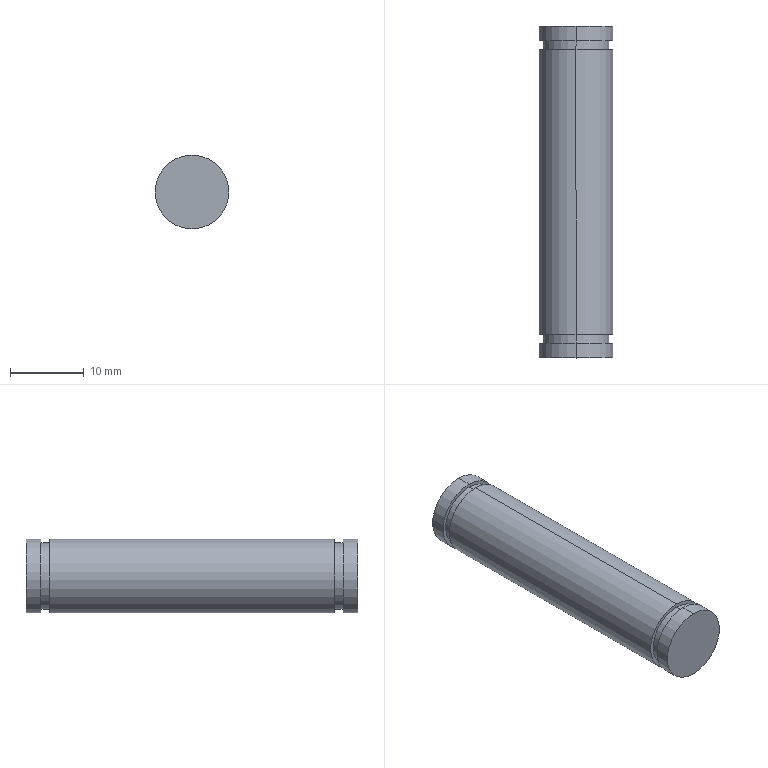Part | SolidWorks | features Revolution 1 | 1 solid | 16 faces | box 10 x 45 x 10 mm | volume 3498 mm3 | cylinder 10 | plane 6 | commonest cylinder face diameters 10 x6 9 x4
STEP:
#1=CARTESIAN_POINT('',(0.,-20.5,4.5));
#2=VERTEX_POINT('',#1);
#3=CARTESIAN_POINT('',(0.,-20.5,-4.5));
#4=VERTEX_POINT('',#3);
#5=CARTESIAN_POINT('',(0.,-20.5,0.));
#6=DIRECTION('',(0.,1.,0.));
#7=DIRECTION('',(0.,0.,1.));
#8=AXIS2_PLACEMENT_3D('',#5,#6,#7);
#9=CIRCLE('',#8,4.5);
#10=EDGE_CURVE('',#2,#4,#9,.T.);
#11=ORIENTED_EDGE('',*,*,#10,.T.);
#12=CARTESIAN_POINT('',(0.,-19.3,-4.5));
#13=VERTEX_POINT('',#12);
#14=CARTESIAN_POINT('',(0.,-22.5,-4.5));
#15=DIRECTION('',(0.,1.,0.));
#16=VECTOR('',#15,1000.);
#17=LINE('',#14,#16);
#18=EDGE_CURVE('',#4,#13,#17,.T.);
#19=ORIENTED_EDGE('',*,*,#18,.T.);
#20=CARTESIAN_POINT('',(0.,-19.3,4.5));
#21=VERTEX_POINT('',#20);
#22=CARTESIAN_POINT('',(0.,-19.3,0.));
#23=DIRECTION('',(0.,1.,0.));
#24=DIRECTION('',(0.,0.,1.));
#25=AXIS2_PLACEMENT_3D('',#22,#23,#24);
#26=CIRCLE('',#25,4.5);
#27=EDGE_CURVE('',#21,#13,#26,.T.);
#28=ORIENTED_EDGE('',*,*,#27,.F.);
#29=CARTESIAN_POINT('',(0.,-22.5,4.5));
#30=DIRECTION('',(0.,1.,0.));
#31=VECTOR('',#30,1000.);
#32=LINE('',#29,#31);
#33=EDGE_CURVE('',#2,#21,#32,.T.);
#34=ORIENTED_EDGE('',*,*,#33,.F.);
#35=EDGE_LOOP('',(#11,#19,#28,#34));
#36=FACE_OUTER_BOUND('',#35,.T.);
#37=CARTESIAN_POINT('',(0.,-22.5,0.));
#38=DIRECTION('',(0.,1.,0.));
#39=DIRECTION('',(0.,0.,1.));
#40=AXIS2_PLACEMENT_3D('',#37,#38,#39);
#41=CYLINDRICAL_SURFACE('',#40,4.5);
#42=ADVANCED_FACE('',(#36),#41,.T.);
#43=CARTESIAN_POINT('',(0.,-19.3,5.));
#44=VERTEX_POINT('',#43);
#45=CARTESIAN_POINT('',(0.,-19.3,-5.));
#46=VERTEX_POINT('',#45);
#47=CARTESIAN_POINT('',(0.,-19.3,0.));
#48=DIRECTION('',(0.,1.,0.));
#49=DIRECTION('',(0.,0.,1.));
#50=AXIS2_PLACEMENT_3D('',#47,#48,#49);
#51=CIRCLE('',#50,5.);
#52=EDGE_CURVE('',#44,#46,#51,.T.);
#53=ORIENTED_EDGE('',*,*,#52,.T.);
#54=CARTESIAN_POINT('',(0.,19.3,-5.));
#55=VERTEX_POINT('',#54);
#56=CARTESIAN_POINT('',(0.,-22.5,-5.));
#57=DIRECTION('',(0.,1.,0.));
#58=VECTOR('',#57,1000.);
#59=LINE('',#56,#58);
#60=EDGE_CURVE('',#46,#55,#59,.T.);
#61=ORIENTED_EDGE('',*,*,#60,.T.);
#62=CARTESIAN_POINT('',(0.,19.3,5.));
#63=VERTEX_POINT('',#62);
#64=CARTESIAN_POINT('',(0.,19.3,0.));
#65=DIRECTION('',(0.,1.,0.));
#66=DIRECTION('',(0.,0.,1.));
#67=AXIS2_PLACEMENT_3D('',#64,#65,#66);
#68=CIRCLE('',#67,5.);
#69=EDGE_CURVE('',#63,#55,#68,.T.);
#70=ORIENTED_EDGE('',*,*,#69,.F.);
#71=CARTESIAN_POINT('',(0.,-22.5,5.));
#72=DIRECTION('',(0.,1.,0.));
#73=VECTOR('',#72,1000.);
#74=LINE('',#71,#73);
#75=EDGE_CURVE('',#44,#63,#74,.T.);
#76=ORIENTED_EDGE('',*,*,#75,.F.);
#77=EDGE_LOOP('',(#53,#61,#70,#76));
#78=FACE_OUTER_BOUND('',#77,.T.);
#79=CARTESIAN_POINT('',(0.,-22.5,0.));
#80=DIRECTION('',(0.,1.,0.));
#81=DIRECTION('',(0.,0.,1.));
#82=AXIS2_PLACEMENT_3D('',#79,#80,#81);
#83=CYLINDRICAL_SURFACE('',#82,5.);
#84=ADVANCED_FACE('',(#78),#83,.T.);
#85=CARTESIAN_POINT('',(0.,19.3,4.5));
#86=VERTEX_POINT('',#85);
#87=CARTESIAN_POINT('',(0.,19.3,-4.5));
#88=VERTEX_POINT('',#87);
#89=CARTESIAN_POINT('',(0.,19.3,0.));
#90=DIRECTION('',(0.,1.,0.));
#91=DIRECTION('',(0.,0.,1.));
#92=AXIS2_PLACEMENT_3D('',#89,#90,#91);
#93=CIRCLE('',#92,4.5);
#94=EDGE_CURVE('',#86,#88,#93,.T.);
#95=ORIENTED_EDGE('',*,*,#94,.T.);
#96=CARTESIAN_POINT('',(0.,20.5,-4.5));
#97=VERTEX_POINT('',#96);
#98=CARTESIAN_POINT('',(0.,-22.5,-4.5));
#99=DIRECTION('',(0.,1.,0.));
#100=VECTOR('',#99,1000.);
#101=LINE('',#98,#100);
#102=EDGE_CURVE('',#88,#97,#101,.T.);
#103=ORIENTED_EDGE('',*,*,#102,.T.);
#104=CARTESIAN_POINT('',(0.,20.5,4.5));
#105=VERTEX_POINT('',#104);
#106=CARTESIAN_POINT('',(0.,20.5,0.));
#107=DIRECTION('',(0.,1.,0.));
#108=DIRECTION('',(0.,0.,1.));
#109=AXIS2_PLACEMENT_3D('',#106,#107,#108);
#110=CIRCLE('',#109,4.5);
#111=EDGE_CURVE('',#105,#97,#110,.T.);
#112=ORIENTED_EDGE('',*,*,#111,.F.);
#113=CARTESIAN_POINT('',(0.,-22.5,4.5));
#114=DIRECTION('',(0.,1.,0.));
#115=VECTOR('',#114,1000.);
#116=LINE('',#113,#115);
#117=EDGE_CURVE('',#86,#105,#116,.T.);
#118=ORIENTED_EDGE('',*,*,#117,.F.);
#119=EDGE_LOOP('',(#95,#103,#112,#118));
#120=FACE_OUTER_BOUND('',#119,.T.);
#121=CARTESIAN_POINT('',(0.,-22.5,0.));
#122=DIRECTION('',(0.,1.,0.));
#123=DIRECTION('',(0.,0.,1.));
#124=AXIS2_PLACEMENT_3D('',#121,#122,#123);
#125=CYLINDRICAL_SURFACE('',#124,4.5);
#126=ADVANCED_FACE('',(#120),#125,.T.);
#127=CARTESIAN_POINT('',(0.,20.5,5.));
#128=VERTEX_POINT('',#127);
#129=CARTESIAN_POINT('',(0.,20.5,-5.));
#130=VERTEX_POINT('',#129);
#131=CARTESIAN_POINT('',(0.,20.5,0.));
#132=DIRECTION('',(0.,1.,0.));
#133=DIRECTION('',(0.,0.,1.));
#134=AXIS2_PLACEMENT_3D('',#131,#132,#133);
#135=CIRCLE('',#134,5.);
#136=EDGE_CURVE('',#128,#130,#135,.T.);
#137=ORIENTED_EDGE('',*,*,#136,.T.);
#138=CARTESIAN_POINT('',(0.,22.5,-5.));
#139=VERTEX_POINT('',#138);
#140=CARTESIAN_POINT('',(0.,-22.5,-5.));
#141=DIRECTION('',(0.,1.,0.));
#142=VECTOR('',#141,1000.);
#143=LINE('',#140,#142);
#144=EDGE_CURVE('',#130,#139,#143,.T.);
#145=ORIENTED_EDGE('',*,*,#144,.T.);
#146=CARTESIAN_POINT('',(0.,22.5,5.));
#147=VERTEX_POINT('',#146);
#148=CARTESIAN_POINT('',(0.,22.5,0.));
#149=DIRECTION('',(0.,1.,0.));
#150=DIRECTION('',(0.,0.,1.));
#151=AXIS2_PLACEMENT_3D('',#148,#149,#150);
#152=CIRCLE('',#151,5.);
#153=EDGE_CURVE('',#147,#139,#152,.T.);
#154=ORIENTED_EDGE('',*,*,#153,.F.);
#155=CARTESIAN_POINT('',(0.,-22.5,5.));
#156=DIRECTION('',(0.,1.,0.));
#157=VECTOR('',#156,1000.);
#158=LINE('',#155,#157);
#159=EDGE_CURVE('',#128,#147,#158,.T.);
#160=ORIENTED_EDGE('',*,*,#159,.F.);
#161=EDGE_LOOP('',(#137,#145,#154,#160));
#162=FACE_OUTER_BOUND('',#161,.T.);
#163=CARTESIAN_POINT('',(0.,-22.5,0.));
#164=DIRECTION('',(0.,1.,0.));
#165=DIRECTION('',(0.,0.,1.));
#166=AXIS2_PLACEMENT_3D('',#163,#164,#165);
#167=CYLINDRICAL_SURFACE('',#166,5.);
#168=ADVANCED_FACE('',(#162),#167,.T.);
#169=CARTESIAN_POINT('',(0.,-22.5,5.));
#170=VERTEX_POINT('',#169);
#171=CARTESIAN_POINT('',(0.,-22.5,-5.));
#172=VERTEX_POINT('',#171);
#173=CARTESIAN_POINT('',(0.,-22.5,0.));
#174=DIRECTION('',(0.,1.,0.));
#175=DIRECTION('',(0.,0.,1.));
#176=AXIS2_PLACEMENT_3D('',#173,#174,#175);
#177=CIRCLE('',#176,5.);
#178=EDGE_CURVE('',#170,#172,#177,.T.);
#179=ORIENTED_EDGE('',*,*,#178,.T.);
#180=CARTESIAN_POINT('',(0.,-20.5,-5.));
#181=VERTEX_POINT('',#180);
#182=CARTESIAN_POINT('',(0.,-22.5,-5.));
#183=DIRECTION('',(0.,1.,0.));
#184=VECTOR('',#183,1000.);
#185=LINE('',#182,#184);
#186=EDGE_CURVE('',#172,#181,#185,.T.);
#187=ORIENTED_EDGE('',*,*,#186,.T.);
#188=CARTESIAN_POINT('',(0.,-20.5,5.));
#189=VERTEX_POINT('',#188);
#190=CARTESIAN_POINT('',(0.,-20.5,0.));
#191=DIRECTION('',(0.,1.,0.));
#192=DIRECTION('',(0.,0.,1.));
#193=AXIS2_PLACEMENT_3D('',#190,#191,#192);
#194=CIRCLE('',#193,5.);
#195=EDGE_CURVE('',#189,#181,#194,.T.);
#196=ORIENTED_EDGE('',*,*,#195,.F.);
#197=CARTESIAN_POINT('',(0.,-22.5,5.));
#198=DIRECTION('',(0.,1.,0.));
#199=VECTOR('',#198,1000.);
#200=LINE('',#197,#199);
#201=EDGE_CURVE('',#170,#189,#200,.T.);
#202=ORIENTED_EDGE('',*,*,#201,.F.);
#203=EDGE_LOOP('',(#179,#187,#196,#202));
#204=FACE_OUTER_BOUND('',#203,.T.);
#205=CARTESIAN_POINT('',(0.,-22.5,0.));
#206=DIRECTION('',(0.,1.,0.));
#207=DIRECTION('',(0.,0.,1.));
#208=AXIS2_PLACEMENT_3D('',#205,#206,#207);
#209=CYLINDRICAL_SURFACE('',#208,5.);
#210=ADVANCED_FACE('',(#204),#209,.T.);
#211=ORIENTED_EDGE('',*,*,#186,.F.);
#212=CARTESIAN_POINT('',(0.,-22.5,0.));
#213=DIRECTION('',(0.,1.,0.));
#214=DIRECTION('',(0.,0.,1.));
#215=AXIS2_PLACEMENT_3D('',#212,#213,#214);
#216=CIRCLE('',#215,5.);
#217=EDGE_CURVE('',#172,#170,#216,.T.);
#218=ORIENTED_EDGE('',*,*,#217,.T.);
#219=ORIENTED_EDGE('',*,*,#201,.T.);
#220=CARTESIAN_POINT('',(0.,-20.5,0.));
#221=DIRECTION('',(0.,1.,0.));
#222=DIRECTION('',(0.,0.,1.));
#223=AXIS2_PLACEMENT_3D('',#220,#221,#222);
#224=CIRCLE('',#223,5.);
#225=EDGE_CURVE('',#181,#189,#224,.T.);
#226=ORIENTED_EDGE('',*,*,#225,.F.);
#227=EDGE_LOOP('',(#211,#218,#219,#226));
#228=FACE_OUTER_BOUND('',#227,.T.);
#229=CARTESIAN_POINT('',(0.,-22.5,0.));
#230=DIRECTION('',(0.,1.,0.));
#231=DIRECTION('',(0.,0.,1.));
#232=AXIS2_PLACEMENT_3D('',#229,#230,#231);
#233=CYLINDRICAL_SURFACE('',#232,5.);
#234=ADVANCED_FACE('',(#228),#233,.T.);
#235=ORIENTED_EDGE('',*,*,#178,.F.);
#236=ORIENTED_EDGE('',*,*,#217,.F.);
#237=EDGE_LOOP('',(#235,#236));
#238=FACE_OUTER_BOUND('',#237,.T.);
#239=CARTESIAN_POINT('',(5.,-22.5,0.));
#240=DIRECTION('',(0.,-1.,0.));
#241=DIRECTION('',(0.,0.,-1.));
#242=AXIS2_PLACEMENT_3D('',#239,#240,#241);
#243=PLANE('',#242);
#244=ADVANCED_FACE('',(#238),#243,.T.);
#245=ORIENTED_EDGE('',*,*,#153,.T.);
#246=CARTESIAN_POINT('',(0.,22.5,0.));
#247=DIRECTION('',(0.,1.,0.));
#248=DIRECTION('',(0.,0.,1.));
#249=AXIS2_PLACEMENT_3D('',#246,#247,#248);
#250=CIRCLE('',#249,5.);
#251=EDGE_CURVE('',#139,#147,#250,.T.);
#252=ORIENTED_EDGE('',*,*,#251,.T.);
#253=EDGE_LOOP('',(#245,#252));
#254=FACE_OUTER_BOUND('',#253,.T.);
#255=CARTESIAN_POINT('',(0.,22.5,0.));
#256=DIRECTION('',(0.,1.,0.));
#257=DIRECTION('',(0.,0.,1.));
#258=AXIS2_PLACEMENT_3D('',#255,#256,#257);
#259=PLANE('',#258);
#260=ADVANCED_FACE('',(#254),#259,.T.);
#261=ORIENTED_EDGE('',*,*,#144,.F.);
#262=CARTESIAN_POINT('',(0.,20.5,0.));
#263=DIRECTION('',(0.,1.,0.));
#264=DIRECTION('',(0.,0.,1.));
#265=AXIS2_PLACEMENT_3D('',#262,#263,#264);
#266=CIRCLE('',#265,5.);
#267=EDGE_CURVE('',#130,#128,#266,.T.);
#268=ORIENTED_EDGE('',*,*,#267,.T.);
#269=ORIENTED_EDGE('',*,*,#159,.T.);
#270=ORIENTED_EDGE('',*,*,#251,.F.);
#271=EDGE_LOOP('',(#261,#268,#269,#270));
#272=FACE_OUTER_BOUND('',#271,.T.);
#273=CARTESIAN_POINT('',(0.,-22.5,0.));
#274=DIRECTION('',(0.,1.,0.));
#275=DIRECTION('',(0.,0.,1.));
#276=AXIS2_PLACEMENT_3D('',#273,#274,#275);
#277=CYLINDRICAL_SURFACE('',#276,5.);
#278=ADVANCED_FACE('',(#272),#277,.T.);
#279=ORIENTED_EDGE('',*,*,#111,.T.);
#280=CARTESIAN_POINT('',(0.,20.5,0.));
#281=DIRECTION('',(0.,1.,0.));
#282=DIRECTION('',(0.,0.,1.));
#283=AXIS2_PLACEMENT_3D('',#280,#281,#282);
#284=CIRCLE('',#283,4.5);
#285=EDGE_CURVE('',#97,#105,#284,.T.);
#286=ORIENTED_EDGE('',*,*,#285,.T.);
#287=EDGE_LOOP('',(#279,#286));
#288=FACE_BOUND('',#287,.T.);
#289=ORIENTED_EDGE('',*,*,#136,.F.);
#290=ORIENTED_EDGE('',*,*,#267,.F.);
#291=EDGE_LOOP('',(#289,#290));
#292=FACE_OUTER_BOUND('',#291,.T.);
#293=CARTESIAN_POINT('',(5.,20.5,0.));
#294=DIRECTION('',(0.,-1.,0.));
#295=DIRECTION('',(0.,0.,-1.));
#296=AXIS2_PLACEMENT_3D('',#293,#294,#295);
#297=PLANE('',#296);
#298=ADVANCED_FACE('',(#288,#292),#297,.T.);
#299=ORIENTED_EDGE('',*,*,#102,.F.);
#300=CARTESIAN_POINT('',(0.,19.3,0.));
#301=DIRECTION('',(0.,1.,0.));
#302=DIRECTION('',(0.,0.,1.));
#303=AXIS2_PLACEMENT_3D('',#300,#301,#302);
#304=CIRCLE('',#303,4.5);
#305=EDGE_CURVE('',#88,#86,#304,.T.);
#306=ORIENTED_EDGE('',*,*,#305,.T.);
#307=ORIENTED_EDGE('',*,*,#117,.T.);
#308=ORIENTED_EDGE('',*,*,#285,.F.);
#309=EDGE_LOOP('',(#299,#306,#307,#308));
#310=FACE_OUTER_BOUND('',#309,.T.);
#311=CARTESIAN_POINT('',(0.,-22.5,0.));
#312=DIRECTION('',(0.,1.,0.));
#313=DIRECTION('',(0.,0.,1.));
#314=AXIS2_PLACEMENT_3D('',#311,#312,#313);
#315=CYLINDRICAL_SURFACE('',#314,4.5);
#316=ADVANCED_FACE('',(#310),#315,.T.);
#317=ORIENTED_EDGE('',*,*,#69,.T.);
#318=CARTESIAN_POINT('',(0.,19.3,0.));
#319=DIRECTION('',(0.,1.,0.));
#320=DIRECTION('',(0.,0.,1.));
#321=AXIS2_PLACEMENT_3D('',#318,#319,#320);
#322=CIRCLE('',#321,5.);
#323=EDGE_CURVE('',#55,#63,#322,.T.);
#324=ORIENTED_EDGE('',*,*,#323,.T.);
#325=EDGE_LOOP('',(#317,#324));
#326=FACE_OUTER_BOUND('',#325,.T.);
#327=ORIENTED_EDGE('',*,*,#94,.F.);
#328=ORIENTED_EDGE('',*,*,#305,.F.);
#329=EDGE_LOOP('',(#327,#328));
#330=FACE_BOUND('',#329,.T.);
#331=CARTESIAN_POINT('',(4.5,19.3,0.));
#332=DIRECTION('',(0.,1.,0.));
#333=DIRECTION('',(0.,0.,1.));
#334=AXIS2_PLACEMENT_3D('',#331,#332,#333);
#335=PLANE('',#334);
#336=ADVANCED_FACE('',(#326,#330),#335,.T.);
#337=ORIENTED_EDGE('',*,*,#60,.F.);
#338=CARTESIAN_POINT('',(0.,-19.3,0.));
#339=DIRECTION('',(0.,1.,0.));
#340=DIRECTION('',(0.,0.,1.));
#341=AXIS2_PLACEMENT_3D('',#338,#339,#340);
#342=CIRCLE('',#341,5.);
#343=EDGE_CURVE('',#46,#44,#342,.T.);
#344=ORIENTED_EDGE('',*,*,#343,.T.);
#345=ORIENTED_EDGE('',*,*,#75,.T.);
#346=ORIENTED_EDGE('',*,*,#323,.F.);
#347=EDGE_LOOP('',(#337,#344,#345,#346));
#348=FACE_OUTER_BOUND('',#347,.T.);
#349=CARTESIAN_POINT('',(0.,-22.5,0.));
#350=DIRECTION('',(0.,1.,0.));
#351=DIRECTION('',(0.,0.,1.));
#352=AXIS2_PLACEMENT_3D('',#349,#350,#351);
#353=CYLINDRICAL_SURFACE('',#352,5.);
#354=ADVANCED_FACE('',(#348),#353,.T.);
#355=ORIENTED_EDGE('',*,*,#27,.T.);
#356=CARTESIAN_POINT('',(0.,-19.3,0.));
#357=DIRECTION('',(0.,1.,0.));
#358=DIRECTION('',(0.,0.,1.));
#359=AXIS2_PLACEMENT_3D('',#356,#357,#358);
#360=CIRCLE('',#359,4.5);
#361=EDGE_CURVE('',#13,#21,#360,.T.);
#362=ORIENTED_EDGE('',*,*,#361,.T.);
#363=EDGE_LOOP('',(#355,#362));
#364=FACE_BOUND('',#363,.T.);
#365=ORIENTED_EDGE('',*,*,#52,.F.);
#366=ORIENTED_EDGE('',*,*,#343,.F.);
#367=EDGE_LOOP('',(#365,#366));
#368=FACE_OUTER_BOUND('',#367,.T.);
#369=CARTESIAN_POINT('',(5.,-19.3,0.));
#370=DIRECTION('',(0.,-1.,0.));
#371=DIRECTION('',(0.,0.,-1.));
#372=AXIS2_PLACEMENT_3D('',#369,#370,#371);
#373=PLANE('',#372);
#374=ADVANCED_FACE('',(#364,#368),#373,.T.);
#375=ORIENTED_EDGE('',*,*,#18,.F.);
#376=CARTESIAN_POINT('',(0.,-20.5,0.));
#377=DIRECTION('',(0.,1.,0.));
#378=DIRECTION('',(0.,0.,1.));
#379=AXIS2_PLACEMENT_3D('',#376,#377,#378);
#380=CIRCLE('',#379,4.5);
#381=EDGE_CURVE('',#4,#2,#380,.T.);
#382=ORIENTED_EDGE('',*,*,#381,.T.);
#383=ORIENTED_EDGE('',*,*,#33,.T.);
#384=ORIENTED_EDGE('',*,*,#361,.F.);
#385=EDGE_LOOP('',(#375,#382,#383,#384));
#386=FACE_OUTER_BOUND('',#385,.T.);
#387=CARTESIAN_POINT('',(0.,-22.5,0.));
#388=DIRECTION('',(0.,1.,0.));
#389=DIRECTION('',(0.,0.,1.));
#390=AXIS2_PLACEMENT_3D('',#387,#388,#389);
#391=CYLINDRICAL_SURFACE('',#390,4.5);
#392=ADVANCED_FACE('',(#386),#391,.T.);
#393=ORIENTED_EDGE('',*,*,#195,.T.);
#394=ORIENTED_EDGE('',*,*,#225,.T.);
#395=EDGE_LOOP('',(#393,#394));
#396=FACE_OUTER_BOUND('',#395,.T.);
#397=ORIENTED_EDGE('',*,*,#10,.F.);
#398=ORIENTED_EDGE('',*,*,#381,.F.);
#399=EDGE_LOOP('',(#397,#398));
#400=FACE_BOUND('',#399,.T.);
#401=CARTESIAN_POINT('',(4.5,-20.5,0.));
#402=DIRECTION('',(0.,1.,0.));
#403=DIRECTION('',(0.,0.,1.));
#404=AXIS2_PLACEMENT_3D('',#401,#402,#403);
#405=PLANE('',#404);
#406=ADVANCED_FACE('',(#396,#400),#405,.T.);
#407=CLOSED_SHELL('',(#42,#84,#126,#168,#210,#234,#244,#260,#278,#298,#316,#336,#354,#374,#392,#406));
#408=MANIFOLD_SOLID_BREP('',#407);
#409=CARTESIAN_POINT('',(0.,0.,0.));
#410=DIRECTION('',(0.,0.,1.));
#411=DIRECTION('',(1.,0.,0.));
#412=AXIS2_PLACEMENT_3D('',#409,#410,#411);
#413=(LENGTH_UNIT()NAMED_UNIT(*)SI_UNIT(.MILLI.,.METRE.));
#414=UNCERTAINTY_MEASURE_WITH_UNIT(LENGTH_MEASURE(0.00001),#413,'','');
#415=(NAMED_UNIT(*)PLANE_ANGLE_UNIT()SI_UNIT($,.RADIAN.));
#416=(NAMED_UNIT(*)SI_UNIT($,.STERADIAN.)SOLID_ANGLE_UNIT());
#417=(GEOMETRIC_REPRESENTATION_CONTEXT(3)GLOBAL_UNCERTAINTY_ASSIGNED_CONTEXT((#414))GLOBAL_UNIT_ASSIGNED_CONTEXT((#413,#415,#416))REPRESENTATION_CONTEXT('',''));
#418=ADVANCED_BREP_SHAPE_REPRESENTATION('',(#408,#412),#417);